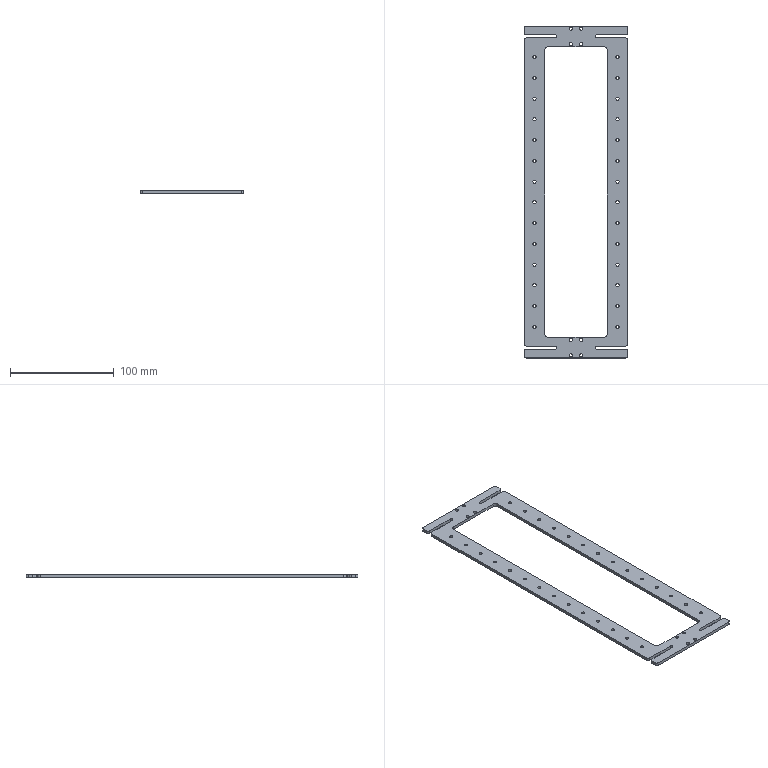Part | SolidWorks | features BaseBody 1 | 1 solid | 116 faces | box 100 x 320 x 3 mm | volume 43656 mm3 | cylinder 94 | plane 22 | commonest cylinder face diameters 3 x56 3.1 x22 4 x12 6 x4